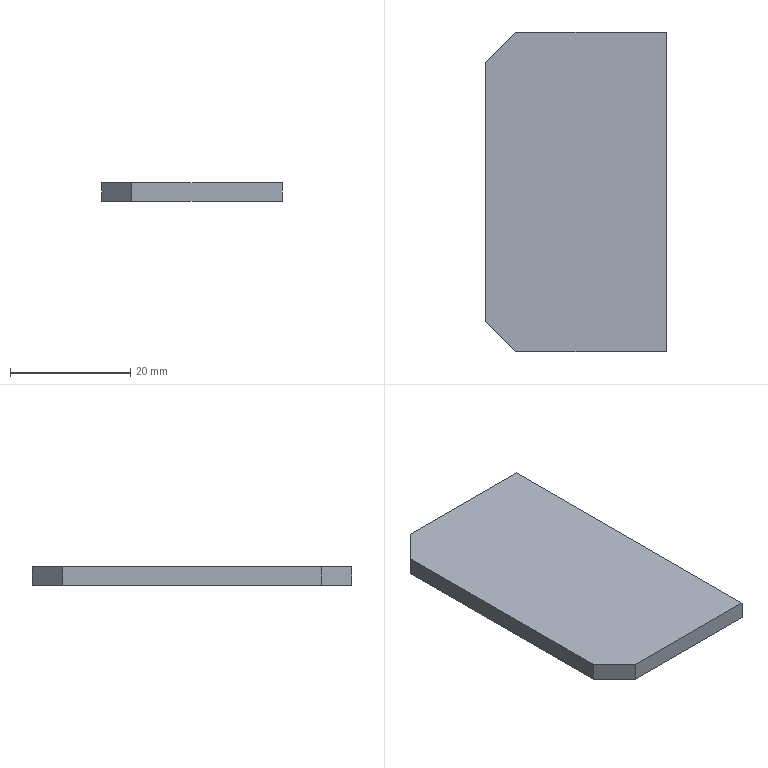Part | SolidWorks | features Chamfer 1, FlatPattern 1, SMBaseFlange 1, SheetMetal 1 | 1 solid | 8 faces | box 30 x 53 x 3 mm | volume 4695 mm3 | plane 8
STEP:
#1=CARTESIAN_POINT('',(30.,26.5,-3.));
#2=VERTEX_POINT('',#1);
#3=CARTESIAN_POINT('',(5.,26.5,-3.));
#4=VERTEX_POINT('',#3);
#5=CARTESIAN_POINT('',(30.,26.5,-3.));
#6=DIRECTION('',(-1.,0.,0.));
#7=VECTOR('',#6,1000.);
#8=LINE('',#5,#7);
#9=EDGE_CURVE('',#2,#4,#8,.T.);
#10=ORIENTED_EDGE('',*,*,#9,.T.);
#11=CARTESIAN_POINT('',(5.,26.5,0.));
#12=VERTEX_POINT('',#11);
#13=CARTESIAN_POINT('',(5.,26.5,-3.));
#14=DIRECTION('',(0.,0.,1.));
#15=VECTOR('',#14,1000.);
#16=LINE('',#13,#15);
#17=EDGE_CURVE('',#4,#12,#16,.T.);
#18=ORIENTED_EDGE('',*,*,#17,.T.);
#19=CARTESIAN_POINT('',(30.,26.5,0.));
#20=VERTEX_POINT('',#19);
#21=CARTESIAN_POINT('',(30.,26.5,0.));
#22=DIRECTION('',(-1.,0.,0.));
#23=VECTOR('',#22,1000.);
#24=LINE('',#21,#23);
#25=EDGE_CURVE('',#20,#12,#24,.T.);
#26=ORIENTED_EDGE('',*,*,#25,.F.);
#27=CARTESIAN_POINT('',(30.,26.5,-3.));
#28=DIRECTION('',(0.,0.,1.));
#29=VECTOR('',#28,1000.);
#30=LINE('',#27,#29);
#31=EDGE_CURVE('',#2,#20,#30,.T.);
#32=ORIENTED_EDGE('',*,*,#31,.F.);
#33=EDGE_LOOP('',(#10,#18,#26,#32));
#34=FACE_OUTER_BOUND('',#33,.T.);
#35=CARTESIAN_POINT('',(30.,26.5,-3.));
#36=DIRECTION('',(0.,1.,0.));
#37=DIRECTION('',(-1.,0.,0.));
#38=AXIS2_PLACEMENT_3D('',#35,#36,#37);
#39=PLANE('',#38);
#40=ADVANCED_FACE('',(#34),#39,.T.);
#41=CARTESIAN_POINT('',(30.,-26.5,0.));
#42=VERTEX_POINT('',#41);
#43=CARTESIAN_POINT('',(30.,-26.5,0.));
#44=DIRECTION('',(0.,1.,0.));
#45=VECTOR('',#44,1000.);
#46=LINE('',#43,#45);
#47=EDGE_CURVE('',#42,#20,#46,.T.);
#48=ORIENTED_EDGE('',*,*,#47,.F.);
#49=CARTESIAN_POINT('',(30.,-26.5,-3.));
#50=VERTEX_POINT('',#49);
#51=CARTESIAN_POINT('',(30.,-26.5,-3.));
#52=DIRECTION('',(0.,0.,1.));
#53=VECTOR('',#52,1000.);
#54=LINE('',#51,#53);
#55=EDGE_CURVE('',#50,#42,#54,.T.);
#56=ORIENTED_EDGE('',*,*,#55,.F.);
#57=CARTESIAN_POINT('',(30.,-26.5,-3.));
#58=DIRECTION('',(0.,1.,0.));
#59=VECTOR('',#58,1000.);
#60=LINE('',#57,#59);
#61=EDGE_CURVE('',#50,#2,#60,.T.);
#62=ORIENTED_EDGE('',*,*,#61,.T.);
#63=ORIENTED_EDGE('',*,*,#31,.T.);
#64=EDGE_LOOP('',(#48,#56,#62,#63));
#65=FACE_OUTER_BOUND('',#64,.T.);
#66=CARTESIAN_POINT('',(30.,-26.5,-3.));
#67=DIRECTION('',(1.,0.,0.));
#68=DIRECTION('',(0.,1.,0.));
#69=AXIS2_PLACEMENT_3D('',#66,#67,#68);
#70=PLANE('',#69);
#71=ADVANCED_FACE('',(#65),#70,.T.);
#72=CARTESIAN_POINT('',(5.,-26.5,0.));
#73=VERTEX_POINT('',#72);
#74=CARTESIAN_POINT('',(0.,-26.5,0.));
#75=DIRECTION('',(1.,0.,0.));
#76=VECTOR('',#75,1000.);
#77=LINE('',#74,#76);
#78=EDGE_CURVE('',#73,#42,#77,.T.);
#79=ORIENTED_EDGE('',*,*,#78,.F.);
#80=CARTESIAN_POINT('',(5.,-26.5,-3.));
#81=VERTEX_POINT('',#80);
#82=CARTESIAN_POINT('',(5.,-26.5,-3.));
#83=DIRECTION('',(0.,0.,-1.));
#84=VECTOR('',#83,1000.);
#85=LINE('',#82,#84);
#86=EDGE_CURVE('',#73,#81,#85,.T.);
#87=ORIENTED_EDGE('',*,*,#86,.T.);
#88=CARTESIAN_POINT('',(0.,-26.5,-3.));
#89=DIRECTION('',(1.,0.,0.));
#90=VECTOR('',#89,1000.);
#91=LINE('',#88,#90);
#92=EDGE_CURVE('',#81,#50,#91,.T.);
#93=ORIENTED_EDGE('',*,*,#92,.T.);
#94=ORIENTED_EDGE('',*,*,#55,.T.);
#95=EDGE_LOOP('',(#79,#87,#93,#94));
#96=FACE_OUTER_BOUND('',#95,.T.);
#97=CARTESIAN_POINT('',(0.,-26.5,-3.));
#98=DIRECTION('',(0.,-1.,0.));
#99=DIRECTION('',(0.,0.,-1.));
#100=AXIS2_PLACEMENT_3D('',#97,#98,#99);
#101=PLANE('',#100);
#102=ADVANCED_FACE('',(#96),#101,.T.);
#103=CARTESIAN_POINT('',(0.,21.5,-3.));
#104=VERTEX_POINT('',#103);
#105=CARTESIAN_POINT('',(0.,-21.5,-3.));
#106=VERTEX_POINT('',#105);
#107=CARTESIAN_POINT('',(0.,26.5,-3.));
#108=DIRECTION('',(0.,-1.,0.));
#109=VECTOR('',#108,1000.);
#110=LINE('',#107,#109);
#111=EDGE_CURVE('',#104,#106,#110,.T.);
#112=ORIENTED_EDGE('',*,*,#111,.T.);
#113=CARTESIAN_POINT('',(0.,-21.5,0.));
#114=VERTEX_POINT('',#113);
#115=CARTESIAN_POINT('',(0.,-21.5,-3.));
#116=DIRECTION('',(0.,0.,1.));
#117=VECTOR('',#116,1000.);
#118=LINE('',#115,#117);
#119=EDGE_CURVE('',#106,#114,#118,.T.);
#120=ORIENTED_EDGE('',*,*,#119,.T.);
#121=CARTESIAN_POINT('',(0.,21.5,0.));
#122=VERTEX_POINT('',#121);
#123=CARTESIAN_POINT('',(0.,26.5,0.));
#124=DIRECTION('',(0.,-1.,0.));
#125=VECTOR('',#124,1000.);
#126=LINE('',#123,#125);
#127=EDGE_CURVE('',#122,#114,#126,.T.);
#128=ORIENTED_EDGE('',*,*,#127,.F.);
#129=CARTESIAN_POINT('',(0.,21.5,-3.));
#130=DIRECTION('',(0.,0.,-1.));
#131=VECTOR('',#130,1000.);
#132=LINE('',#129,#131);
#133=EDGE_CURVE('',#122,#104,#132,.T.);
#134=ORIENTED_EDGE('',*,*,#133,.T.);
#135=EDGE_LOOP('',(#112,#120,#128,#134));
#136=FACE_OUTER_BOUND('',#135,.T.);
#137=CARTESIAN_POINT('',(0.,26.5,-3.));
#138=DIRECTION('',(-1.,0.,0.));
#139=DIRECTION('',(0.,-1.,0.));
#140=AXIS2_PLACEMENT_3D('',#137,#138,#139);
#141=PLANE('',#140);
#142=ADVANCED_FACE('',(#136),#141,.T.);
#143=ORIENTED_EDGE('',*,*,#92,.F.);
#144=CARTESIAN_POINT('',(0.,-21.5,-3.));
#145=DIRECTION('',(-0.7071,0.7071,0.));
#146=VECTOR('',#145,1000.);
#147=LINE('',#144,#146);
#148=EDGE_CURVE('',#81,#106,#147,.T.);
#149=ORIENTED_EDGE('',*,*,#148,.T.);
#150=ORIENTED_EDGE('',*,*,#111,.F.);
#151=CARTESIAN_POINT('',(5.,26.5,-3.));
#152=DIRECTION('',(0.7071,0.7071,0.));
#153=VECTOR('',#152,1000.);
#154=LINE('',#151,#153);
#155=EDGE_CURVE('',#104,#4,#154,.T.);
#156=ORIENTED_EDGE('',*,*,#155,.T.);
#157=ORIENTED_EDGE('',*,*,#9,.F.);
#158=ORIENTED_EDGE('',*,*,#61,.F.);
#159=EDGE_LOOP('',(#143,#149,#150,#156,#157,#158));
#160=FACE_OUTER_BOUND('',#159,.T.);
#161=CARTESIAN_POINT('',(0.,0.,-3.));
#162=DIRECTION('',(0.,0.,1.));
#163=DIRECTION('',(1.,0.,0.));
#164=AXIS2_PLACEMENT_3D('',#161,#162,#163);
#165=PLANE('',#164);
#166=ADVANCED_FACE('',(#160),#165,.F.);
#167=ORIENTED_EDGE('',*,*,#127,.T.);
#168=CARTESIAN_POINT('',(-10.75,-10.75,0.));
#169=DIRECTION('',(0.7071,-0.7071,0.));
#170=VECTOR('',#169,1000.);
#171=LINE('',#168,#170);
#172=EDGE_CURVE('',#114,#73,#171,.T.);
#173=ORIENTED_EDGE('',*,*,#172,.T.);
#174=ORIENTED_EDGE('',*,*,#78,.T.);
#175=ORIENTED_EDGE('',*,*,#47,.T.);
#176=ORIENTED_EDGE('',*,*,#25,.T.);
#177=CARTESIAN_POINT('',(-10.75,10.75,0.));
#178=DIRECTION('',(-0.7071,-0.7071,0.));
#179=VECTOR('',#178,1000.);
#180=LINE('',#177,#179);
#181=EDGE_CURVE('',#12,#122,#180,.T.);
#182=ORIENTED_EDGE('',*,*,#181,.T.);
#183=EDGE_LOOP('',(#167,#173,#174,#175,#176,#182));
#184=FACE_OUTER_BOUND('',#183,.T.);
#185=CARTESIAN_POINT('',(0.,0.,0.));
#186=DIRECTION('',(0.,0.,1.));
#187=DIRECTION('',(1.,0.,0.));
#188=AXIS2_PLACEMENT_3D('',#185,#186,#187);
#189=PLANE('',#188);
#190=ADVANCED_FACE('',(#184),#189,.T.);
#191=ORIENTED_EDGE('',*,*,#148,.F.);
#192=ORIENTED_EDGE('',*,*,#86,.F.);
#193=ORIENTED_EDGE('',*,*,#172,.F.);
#194=ORIENTED_EDGE('',*,*,#119,.F.);
#195=EDGE_LOOP('',(#191,#192,#193,#194));
#196=FACE_OUTER_BOUND('',#195,.T.);
#197=CARTESIAN_POINT('',(0.,-21.5,-3.));
#198=DIRECTION('',(0.7071,0.7071,0.));
#199=DIRECTION('',(0.,0.,1.));
#200=AXIS2_PLACEMENT_3D('',#197,#198,#199);
#201=PLANE('',#200);
#202=ADVANCED_FACE('',(#196),#201,.F.);
#203=ORIENTED_EDGE('',*,*,#155,.F.);
#204=ORIENTED_EDGE('',*,*,#133,.F.);
#205=ORIENTED_EDGE('',*,*,#181,.F.);
#206=ORIENTED_EDGE('',*,*,#17,.F.);
#207=EDGE_LOOP('',(#203,#204,#205,#206));
#208=FACE_OUTER_BOUND('',#207,.T.);
#209=CARTESIAN_POINT('',(5.,26.5,-3.));
#210=DIRECTION('',(0.7071,-0.7071,0.));
#211=DIRECTION('',(0.,0.,1.));
#212=AXIS2_PLACEMENT_3D('',#209,#210,#211);
#213=PLANE('',#212);
#214=ADVANCED_FACE('',(#208),#213,.F.);
#215=CLOSED_SHELL('',(#40,#71,#102,#142,#166,#190,#202,#214));
#216=MANIFOLD_SOLID_BREP('',#215);
#217=CARTESIAN_POINT('',(0.,0.,0.));
#218=DIRECTION('',(0.,0.,1.));
#219=DIRECTION('',(1.,0.,0.));
#220=AXIS2_PLACEMENT_3D('',#217,#218,#219);
#221=(LENGTH_UNIT()NAMED_UNIT(*)SI_UNIT(.MILLI.,.METRE.));
#222=UNCERTAINTY_MEASURE_WITH_UNIT(LENGTH_MEASURE(0.00001),#221,'','');
#223=(NAMED_UNIT(*)PLANE_ANGLE_UNIT()SI_UNIT($,.RADIAN.));
#224=(NAMED_UNIT(*)SI_UNIT($,.STERADIAN.)SOLID_ANGLE_UNIT());
#225=(GEOMETRIC_REPRESENTATION_CONTEXT(3)GLOBAL_UNCERTAINTY_ASSIGNED_CONTEXT((#222))GLOBAL_UNIT_ASSIGNED_CONTEXT((#221,#223,#224))REPRESENTATION_CONTEXT('',''));
#226=ADVANCED_BREP_SHAPE_REPRESENTATION('',(#216,#220),#225);